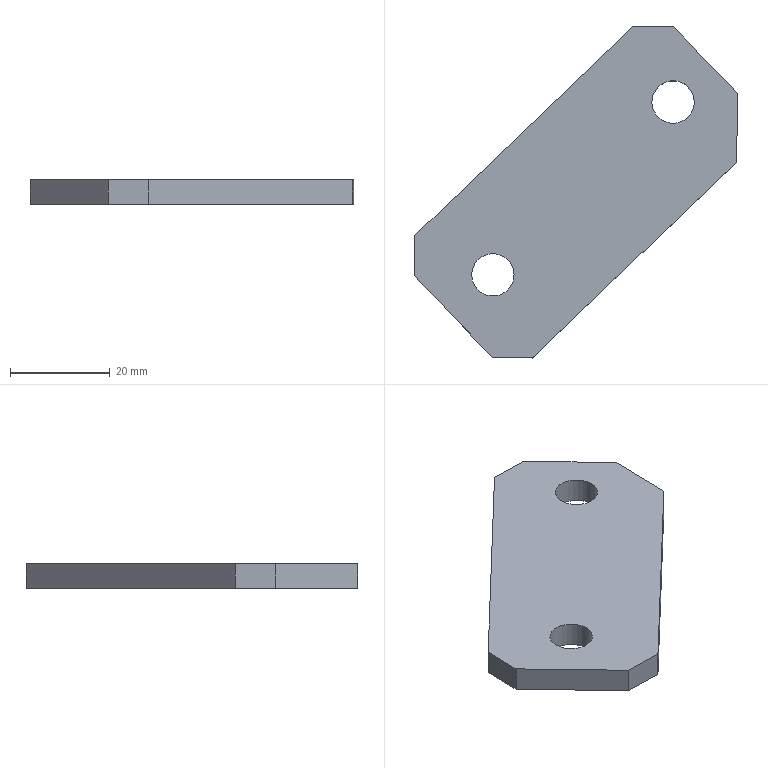Part | STEP file | gslz 2016.10.28-13_id1686_x_t | 1 solid | 12 faces | box 64.831 x 66.474 x 5 mm | volume 11193 mm3 | plane 10 | cylinder 2 | commonest cylinder face diameters 8.5 x2
STEP:
#1=CARTESIAN_POINT('',(0.,0.,0.));
#2=DIRECTION('',(0.,0.,1.));
#3=DIRECTION('',(1.,0.,0.));
#4=AXIS2_PLACEMENT_3D('',#1,#2,#3);
#5=CARTESIAN_POINT('',(590.854,-232.226,-99.));
#6=VERTEX_POINT('',#5);
#7=CARTESIAN_POINT('',(634.582,-190.292,-99.));
#8=VERTEX_POINT('',#7);
#9=CARTESIAN_POINT('',(426.204,-390.12,-99.));
#10=DIRECTION('',(0.7218,0.6921,0.));
#11=VECTOR('',#10,1.);
#12=LINE('',#9,#11);
#13=CARTESIAN_POINT('',(426.204,-390.12,-99.));
#14=DIRECTION('',(0.6921,-0.7218,0.));
#15=DIRECTION('',(0.7218,0.6921,0.));
#16=AXIS2_PLACEMENT_3D('',#13,#14,#15);
#17=PLANE('',#16);
#18=CARTESIAN_POINT('',(0.,0.));
#19=DIRECTION('',(1.,0.));
#20=VECTOR('',#19,1.);
#21=LINE('',#18,#20);
#22=(GEOMETRIC_REPRESENTATION_CONTEXT(2)PARAMETRIC_REPRESENTATION_CONTEXT()REPRESENTATION_CONTEXT('',''));
#23=DEFINITIONAL_REPRESENTATION('',(#21),#22);
#24=PCURVE('',#17,#23);
#25=CARTESIAN_POINT('',(467.733,-433.425,-99.));
#26=DIRECTION('',(0.,0.,1.));
#27=DIRECTION('',(1.,0.,0.));
#28=AXIS2_PLACEMENT_3D('',#25,#26,#27);
#29=PLANE('',#28);
#30=CARTESIAN_POINT('',(-41.529,43.306));
#31=DIRECTION('',(0.7218,0.6921));
#32=VECTOR('',#31,1.);
#33=LINE('',#30,#32);
#34=(GEOMETRIC_REPRESENTATION_CONTEXT(2)PARAMETRIC_REPRESENTATION_CONTEXT()REPRESENTATION_CONTEXT('',''));
#35=DEFINITIONAL_REPRESENTATION('',(#33),#34);
#36=PCURVE('',#29,#35);
#37=SURFACE_CURVE('',#12,(#24,#36),.PCURVE_S1.);
#38=EDGE_CURVE('',#6,#8,#37,.T.);
#39=ORIENTED_EDGE('',*,*,#38,.F.);
#40=CARTESIAN_POINT('',(590.854,-232.226,-94.));
#41=VERTEX_POINT('',#40);
#42=CARTESIAN_POINT('',(590.854,-232.226,-99.));
#43=DIRECTION('',(0.,0.,1.));
#44=VECTOR('',#43,1.);
#45=LINE('',#42,#44);
#46=CARTESIAN_POINT('',(228.122,0.));
#47=DIRECTION('',(0.,1.));
#48=VECTOR('',#47,1.);
#49=LINE('',#46,#48);
#50=(GEOMETRIC_REPRESENTATION_CONTEXT(2)PARAMETRIC_REPRESENTATION_CONTEXT()REPRESENTATION_CONTEXT('',''));
#51=DEFINITIONAL_REPRESENTATION('',(#49),#50);
#52=PCURVE('',#17,#51);
#53=CARTESIAN_POINT('',(590.858,-232.019,-99.));
#54=DIRECTION('',(0.9998,-0.02094,0.));
#55=DIRECTION('',(0.,0.,1.));
#56=AXIS2_PLACEMENT_3D('',#53,#54,#55);
#57=PLANE('',#56);
#58=CARTESIAN_POINT('',(0.,0.2071));
#59=DIRECTION('',(1.,0.));
#60=VECTOR('',#59,1.);
#61=LINE('',#58,#60);
#62=(GEOMETRIC_REPRESENTATION_CONTEXT(2)PARAMETRIC_REPRESENTATION_CONTEXT()REPRESENTATION_CONTEXT('',''));
#63=DEFINITIONAL_REPRESENTATION('',(#61),#62);
#64=PCURVE('',#57,#63);
#65=SURFACE_CURVE('',#45,(#52,#64),.PCURVE_S1.);
#66=EDGE_CURVE('',#6,#41,#65,.T.);
#67=ORIENTED_EDGE('',*,*,#66,.T.);
#68=CARTESIAN_POINT('',(634.582,-190.292,-94.));
#69=VERTEX_POINT('',#68);
#70=CARTESIAN_POINT('',(426.204,-390.12,-94.));
#71=DIRECTION('',(0.7218,0.6921,0.));
#72=VECTOR('',#71,1.);
#73=LINE('',#70,#72);
#74=CARTESIAN_POINT('',(0.,5.));
#75=DIRECTION('',(1.,0.));
#76=VECTOR('',#75,1.);
#77=LINE('',#74,#76);
#78=(GEOMETRIC_REPRESENTATION_CONTEXT(2)PARAMETRIC_REPRESENTATION_CONTEXT()REPRESENTATION_CONTEXT('',''));
#79=DEFINITIONAL_REPRESENTATION('',(#77),#78);
#80=PCURVE('',#17,#79);
#81=CARTESIAN_POINT('',(467.733,-433.425,-94.));
#82=DIRECTION('',(0.,0.,1.));
#83=DIRECTION('',(1.,0.,0.));
#84=AXIS2_PLACEMENT_3D('',#81,#82,#83);
#85=PLANE('',#84);
#86=CARTESIAN_POINT('',(-41.529,43.306));
#87=DIRECTION('',(0.7218,0.6921));
#88=VECTOR('',#87,1.);
#89=LINE('',#86,#88);
#90=(GEOMETRIC_REPRESENTATION_CONTEXT(2)PARAMETRIC_REPRESENTATION_CONTEXT()REPRESENTATION_CONTEXT('',''));
#91=DEFINITIONAL_REPRESENTATION('',(#89),#90);
#92=PCURVE('',#85,#91);
#93=SURFACE_CURVE('',#73,(#80,#92),.PCURVE_S1.);
#94=EDGE_CURVE('',#41,#69,#93,.T.);
#95=ORIENTED_EDGE('',*,*,#94,.T.);
#96=CARTESIAN_POINT('',(634.582,-190.292,-99.));
#97=DIRECTION('',(0.,0.,-1.));
#98=VECTOR('',#97,1.);
#99=LINE('',#96,#98);
#100=CARTESIAN_POINT('',(288.708,0.));
#101=DIRECTION('',(0.,-1.));
#102=VECTOR('',#101,1.);
#103=LINE('',#100,#102);
#104=(GEOMETRIC_REPRESENTATION_CONTEXT(2)PARAMETRIC_REPRESENTATION_CONTEXT()REPRESENTATION_CONTEXT('',''));
#105=DEFINITIONAL_REPRESENTATION('',(#103),#104);
#106=PCURVE('',#17,#105);
#107=CARTESIAN_POINT('',(642.859,-190.466,-99.));
#108=DIRECTION('',(0.02094,0.9998,0.));
#109=DIRECTION('',(0.,0.,-1.));
#110=AXIS2_PLACEMENT_3D('',#107,#108,#109);
#111=PLANE('',#110);
#112=CARTESIAN_POINT('',(0.,8.278));
#113=DIRECTION('',(1.,0.));
#114=VECTOR('',#113,1.);
#115=LINE('',#112,#114);
#116=(GEOMETRIC_REPRESENTATION_CONTEXT(2)PARAMETRIC_REPRESENTATION_CONTEXT()REPRESENTATION_CONTEXT('',''));
#117=DEFINITIONAL_REPRESENTATION('',(#115),#116);
#118=PCURVE('',#111,#117);
#119=SURFACE_CURVE('',#99,(#106,#118),.PCURVE_S1.);
#120=EDGE_CURVE('',#69,#8,#119,.T.);
#121=ORIENTED_EDGE('',*,*,#120,.T.);
#122=EDGE_LOOP('',(#39,#67,#95,#121));
#123=FACE_BOUND('',#122,.T.);
#124=ADVANCED_FACE('',(#123),#17,.F.);
#125=CARTESIAN_POINT('',(655.516,-203.876,-94.));
#126=VERTEX_POINT('',#125);
#127=CARTESIAN_POINT('',(642.652,-190.461,-94.));
#128=VERTEX_POINT('',#127);
#129=CARTESIAN_POINT('',(680.23,-229.648,-94.));
#130=DIRECTION('',(-0.6921,0.7218,0.));
#131=VECTOR('',#130,1.);
#132=LINE('',#129,#131);
#133=CARTESIAN_POINT('',(680.23,-229.648,-99.));
#134=DIRECTION('',(0.7218,0.6921,0.));
#135=DIRECTION('',(-0.6921,0.7218,0.));
#136=AXIS2_PLACEMENT_3D('',#133,#134,#135);
#137=PLANE('',#136);
#138=CARTESIAN_POINT('',(0.,5.));
#139=DIRECTION('',(1.,0.));
#140=VECTOR('',#139,1.);
#141=LINE('',#138,#140);
#142=(GEOMETRIC_REPRESENTATION_CONTEXT(2)PARAMETRIC_REPRESENTATION_CONTEXT()REPRESENTATION_CONTEXT('',''));
#143=DEFINITIONAL_REPRESENTATION('',(#141),#142);
#144=PCURVE('',#137,#143);
#145=CARTESIAN_POINT('',(212.497,203.778));
#146=DIRECTION('',(-0.6921,0.7218));
#147=VECTOR('',#146,1.);
#148=LINE('',#145,#147);
#149=(GEOMETRIC_REPRESENTATION_CONTEXT(2)PARAMETRIC_REPRESENTATION_CONTEXT()REPRESENTATION_CONTEXT('',''));
#150=DEFINITIONAL_REPRESENTATION('',(#148),#149);
#151=PCURVE('',#85,#150);
#152=SURFACE_CURVE('',#132,(#144,#151),.PCURVE_S1.);
#153=EDGE_CURVE('',#126,#128,#152,.T.);
#154=ORIENTED_EDGE('',*,*,#153,.F.);
#155=CARTESIAN_POINT('',(655.516,-203.876,-99.));
#156=VERTEX_POINT('',#155);
#157=CARTESIAN_POINT('',(655.516,-203.876,-99.));
#158=DIRECTION('',(0.,0.,-1.));
#159=VECTOR('',#158,1.);
#160=LINE('',#157,#159);
#161=CARTESIAN_POINT('',(35.707,0.));
#162=DIRECTION('',(0.,-1.));
#163=VECTOR('',#162,1.);
#164=LINE('',#161,#163);
#165=(GEOMETRIC_REPRESENTATION_CONTEXT(2)PARAMETRIC_REPRESENTATION_CONTEXT()REPRESENTATION_CONTEXT('',''));
#166=DEFINITIONAL_REPRESENTATION('',(#164),#165);
#167=PCURVE('',#137,#166);
#168=CARTESIAN_POINT('',(655.224,-217.808,-99.));
#169=DIRECTION('',(-0.9998,0.02094,0.));
#170=DIRECTION('',(0.,0.,1.));
#171=AXIS2_PLACEMENT_3D('',#168,#169,#170);
#172=PLANE('',#171);
#173=CARTESIAN_POINT('',(0.,13.935));
#174=DIRECTION('',(-1.,0.));
#175=VECTOR('',#174,1.);
#176=LINE('',#173,#175);
#177=(GEOMETRIC_REPRESENTATION_CONTEXT(2)PARAMETRIC_REPRESENTATION_CONTEXT()REPRESENTATION_CONTEXT('',''));
#178=DEFINITIONAL_REPRESENTATION('',(#176),#177);
#179=PCURVE('',#172,#178);
#180=SURFACE_CURVE('',#160,(#167,#179),.PCURVE_S1.);
#181=EDGE_CURVE('',#126,#156,#180,.T.);
#182=ORIENTED_EDGE('',*,*,#181,.T.);
#183=CARTESIAN_POINT('',(642.652,-190.461,-99.));
#184=VERTEX_POINT('',#183);
#185=CARTESIAN_POINT('',(680.23,-229.648,-99.));
#186=DIRECTION('',(-0.6921,0.7218,0.));
#187=VECTOR('',#186,1.);
#188=LINE('',#185,#187);
#189=CARTESIAN_POINT('',(0.,0.));
#190=DIRECTION('',(1.,0.));
#191=VECTOR('',#190,1.);
#192=LINE('',#189,#191);
#193=(GEOMETRIC_REPRESENTATION_CONTEXT(2)PARAMETRIC_REPRESENTATION_CONTEXT()REPRESENTATION_CONTEXT('',''));
#194=DEFINITIONAL_REPRESENTATION('',(#192),#193);
#195=PCURVE('',#137,#194);
#196=CARTESIAN_POINT('',(212.497,203.778));
#197=DIRECTION('',(-0.6921,0.7218));
#198=VECTOR('',#197,1.);
#199=LINE('',#196,#198);
#200=(GEOMETRIC_REPRESENTATION_CONTEXT(2)PARAMETRIC_REPRESENTATION_CONTEXT()REPRESENTATION_CONTEXT('',''));
#201=DEFINITIONAL_REPRESENTATION('',(#199),#200);
#202=PCURVE('',#29,#201);
#203=SURFACE_CURVE('',#188,(#195,#202),.PCURVE_S1.);
#204=EDGE_CURVE('',#156,#184,#203,.T.);
#205=ORIENTED_EDGE('',*,*,#204,.T.);
#206=CARTESIAN_POINT('',(642.652,-190.461,-99.));
#207=DIRECTION('',(0.,0.,1.));
#208=VECTOR('',#207,1.);
#209=LINE('',#206,#208);
#210=CARTESIAN_POINT('',(54.293,0.));
#211=DIRECTION('',(0.,1.));
#212=VECTOR('',#211,1.);
#213=LINE('',#210,#212);
#214=(GEOMETRIC_REPRESENTATION_CONTEXT(2)PARAMETRIC_REPRESENTATION_CONTEXT()REPRESENTATION_CONTEXT('',''));
#215=DEFINITIONAL_REPRESENTATION('',(#213),#214);
#216=PCURVE('',#137,#215);
#217=CARTESIAN_POINT('',(0.,0.2071));
#218=DIRECTION('',(-1.,0.));
#219=VECTOR('',#218,1.);
#220=LINE('',#217,#219);
#221=(GEOMETRIC_REPRESENTATION_CONTEXT(2)PARAMETRIC_REPRESENTATION_CONTEXT()REPRESENTATION_CONTEXT('',''));
#222=DEFINITIONAL_REPRESENTATION('',(#220),#221);
#223=PCURVE('',#111,#222);
#224=SURFACE_CURVE('',#209,(#216,#223),.PCURVE_S1.);
#225=EDGE_CURVE('',#184,#128,#224,.T.);
#226=ORIENTED_EDGE('',*,*,#225,.T.);
#227=EDGE_LOOP('',(#154,#182,#205,#226));
#228=FACE_BOUND('',#227,.T.);
#229=ADVANCED_FACE('',(#228),#137,.T.);
#230=CARTESIAN_POINT('',(614.387,-256.766,-99.));
#231=VERTEX_POINT('',#230);
#232=CARTESIAN_POINT('',(655.228,-217.601,-99.));
#233=VERTEX_POINT('',#232);
#234=CARTESIAN_POINT('',(449.737,-414.659,-99.));
#235=DIRECTION('',(0.7218,0.6921,0.));
#236=VECTOR('',#235,1.);
#237=LINE('',#234,#236);
#238=CARTESIAN_POINT('',(449.737,-414.659,-99.));
#239=DIRECTION('',(0.6921,-0.7218,0.));
#240=DIRECTION('',(0.7218,0.6921,0.));
#241=AXIS2_PLACEMENT_3D('',#238,#239,#240);
#242=PLANE('',#241);
#243=CARTESIAN_POINT('',(0.,0.));
#244=DIRECTION('',(1.,0.));
#245=VECTOR('',#244,1.);
#246=LINE('',#243,#245);
#247=(GEOMETRIC_REPRESENTATION_CONTEXT(2)PARAMETRIC_REPRESENTATION_CONTEXT()REPRESENTATION_CONTEXT('',''));
#248=DEFINITIONAL_REPRESENTATION('',(#246),#247);
#249=PCURVE('',#242,#248);
#250=CARTESIAN_POINT('',(-17.996,18.766));
#251=DIRECTION('',(0.7218,0.6921));
#252=VECTOR('',#251,1.);
#253=LINE('',#250,#252);
#254=(GEOMETRIC_REPRESENTATION_CONTEXT(2)PARAMETRIC_REPRESENTATION_CONTEXT()REPRESENTATION_CONTEXT('',''));
#255=DEFINITIONAL_REPRESENTATION('',(#253),#254);
#256=PCURVE('',#29,#255);
#257=SURFACE_CURVE('',#237,(#249,#256),.PCURVE_S1.);
#258=EDGE_CURVE('',#231,#233,#257,.T.);
#259=ORIENTED_EDGE('',*,*,#258,.T.);
#260=CARTESIAN_POINT('',(655.228,-217.601,-94.));
#261=VERTEX_POINT('',#260);
#262=CARTESIAN_POINT('',(655.228,-217.601,-99.));
#263=DIRECTION('',(0.,0.,1.));
#264=VECTOR('',#263,1.);
#265=LINE('',#262,#264);
#266=CARTESIAN_POINT('',(284.708,0.));
#267=DIRECTION('',(0.,1.));
#268=VECTOR('',#267,1.);
#269=LINE('',#266,#268);
#270=(GEOMETRIC_REPRESENTATION_CONTEXT(2)PARAMETRIC_REPRESENTATION_CONTEXT()REPRESENTATION_CONTEXT('',''));
#271=DEFINITIONAL_REPRESENTATION('',(#269),#270);
#272=PCURVE('',#242,#271);
#273=CARTESIAN_POINT('',(0.,0.2071));
#274=DIRECTION('',(1.,0.));
#275=VECTOR('',#274,1.);
#276=LINE('',#273,#275);
#277=(GEOMETRIC_REPRESENTATION_CONTEXT(2)PARAMETRIC_REPRESENTATION_CONTEXT()REPRESENTATION_CONTEXT('',''));
#278=DEFINITIONAL_REPRESENTATION('',(#276),#277);
#279=PCURVE('',#172,#278);
#280=SURFACE_CURVE('',#265,(#272,#279),.PCURVE_S1.);
#281=EDGE_CURVE('',#233,#261,#280,.T.);
#282=ORIENTED_EDGE('',*,*,#281,.T.);
#283=CARTESIAN_POINT('',(614.387,-256.766,-94.));
#284=VERTEX_POINT('',#283);
#285=CARTESIAN_POINT('',(449.737,-414.659,-94.));
#286=DIRECTION('',(0.7218,0.6921,0.));
#287=VECTOR('',#286,1.);
#288=LINE('',#285,#287);
#289=CARTESIAN_POINT('',(0.,5.));
#290=DIRECTION('',(1.,0.));
#291=VECTOR('',#290,1.);
#292=LINE('',#289,#291);
#293=(GEOMETRIC_REPRESENTATION_CONTEXT(2)PARAMETRIC_REPRESENTATION_CONTEXT()REPRESENTATION_CONTEXT('',''));
#294=DEFINITIONAL_REPRESENTATION('',(#292),#293);
#295=PCURVE('',#242,#294);
#296=CARTESIAN_POINT('',(-17.996,18.766));
#297=DIRECTION('',(0.7218,0.6921));
#298=VECTOR('',#297,1.);
#299=LINE('',#296,#298);
#300=(GEOMETRIC_REPRESENTATION_CONTEXT(2)PARAMETRIC_REPRESENTATION_CONTEXT()REPRESENTATION_CONTEXT('',''));
#301=DEFINITIONAL_REPRESENTATION('',(#299),#300);
#302=PCURVE('',#85,#301);
#303=SURFACE_CURVE('',#288,(#295,#302),.PCURVE_S1.);
#304=EDGE_CURVE('',#284,#261,#303,.T.);
#305=ORIENTED_EDGE('',*,*,#304,.F.);
#306=CARTESIAN_POINT('',(614.387,-256.766,-99.));
#307=DIRECTION('',(0.,0.,-1.));
#308=VECTOR('',#307,1.);
#309=LINE('',#306,#308);
#310=CARTESIAN_POINT('',(228.122,0.));
#311=DIRECTION('',(0.,-1.));
#312=VECTOR('',#311,1.);
#313=LINE('',#310,#312);
#314=(GEOMETRIC_REPRESENTATION_CONTEXT(2)PARAMETRIC_REPRESENTATION_CONTEXT()REPRESENTATION_CONTEXT('',''));
#315=DEFINITIONAL_REPRESENTATION('',(#313),#314);
#316=PCURVE('',#242,#315);
#317=CARTESIAN_POINT('',(606.11,-256.593,-99.));
#318=DIRECTION('',(-0.02094,-0.9998,0.));
#319=DIRECTION('',(0.,0.,-1.));
#320=AXIS2_PLACEMENT_3D('',#317,#318,#319);
#321=PLANE('',#320);
#322=CARTESIAN_POINT('',(0.,8.278));
#323=DIRECTION('',(1.,0.));
#324=VECTOR('',#323,1.);
#325=LINE('',#322,#324);
#326=(GEOMETRIC_REPRESENTATION_CONTEXT(2)PARAMETRIC_REPRESENTATION_CONTEXT()REPRESENTATION_CONTEXT('',''));
#327=DEFINITIONAL_REPRESENTATION('',(#325),#326);
#328=PCURVE('',#321,#327);
#329=SURFACE_CURVE('',#309,(#316,#328),.PCURVE_S1.);
#330=EDGE_CURVE('',#284,#231,#329,.T.);
#331=ORIENTED_EDGE('',*,*,#330,.T.);
#332=EDGE_LOOP('',(#259,#282,#305,#331));
#333=FACE_BOUND('',#332,.T.);
#334=ADVANCED_FACE('',(#333),#242,.T.);
#335=CARTESIAN_POINT('',(606.318,-256.597,-99.));
#336=VERTEX_POINT('',#335);
#337=CARTESIAN_POINT('',(590.685,-240.296,-99.));
#338=VERTEX_POINT('',#337);
#339=CARTESIAN_POINT('',(628.263,-279.482,-99.));
#340=DIRECTION('',(-0.6921,0.7218,0.));
#341=VECTOR('',#340,1.);
#342=LINE('',#339,#341);
#343=CARTESIAN_POINT('',(628.263,-279.482,-99.));
#344=DIRECTION('',(0.7218,0.6921,0.));
#345=DIRECTION('',(-0.6921,0.7218,0.));
#346=AXIS2_PLACEMENT_3D('',#343,#344,#345);
#347=PLANE('',#346);
#348=CARTESIAN_POINT('',(0.,0.));
#349=DIRECTION('',(1.,0.));
#350=VECTOR('',#349,1.);
#351=LINE('',#348,#350);
#352=(GEOMETRIC_REPRESENTATION_CONTEXT(2)PARAMETRIC_REPRESENTATION_CONTEXT()REPRESENTATION_CONTEXT('',''));
#353=DEFINITIONAL_REPRESENTATION('',(#351),#352);
#354=PCURVE('',#347,#353);
#355=CARTESIAN_POINT('',(160.531,153.943));
#356=DIRECTION('',(-0.6921,0.7218));
#357=VECTOR('',#356,1.);
#358=LINE('',#355,#357);
#359=(GEOMETRIC_REPRESENTATION_CONTEXT(2)PARAMETRIC_REPRESENTATION_CONTEXT()REPRESENTATION_CONTEXT('',''));
#360=DEFINITIONAL_REPRESENTATION('',(#358),#359);
#361=PCURVE('',#29,#360);
#362=SURFACE_CURVE('',#342,(#354,#361),.PCURVE_S1.);
#363=EDGE_CURVE('',#336,#338,#362,.T.);
#364=ORIENTED_EDGE('',*,*,#363,.F.);
#365=CARTESIAN_POINT('',(606.318,-256.597,-94.));
#366=VERTEX_POINT('',#365);
#367=CARTESIAN_POINT('',(606.318,-256.597,-99.));
#368=DIRECTION('',(0.,0.,1.));
#369=VECTOR('',#368,1.);
#370=LINE('',#367,#369);
#371=CARTESIAN_POINT('',(31.707,0.));
#372=DIRECTION('',(0.,1.));
#373=VECTOR('',#372,1.);
#374=LINE('',#371,#373);
#375=(GEOMETRIC_REPRESENTATION_CONTEXT(2)PARAMETRIC_REPRESENTATION_CONTEXT()REPRESENTATION_CONTEXT('',''));
#376=DEFINITIONAL_REPRESENTATION('',(#374),#375);
#377=PCURVE('',#347,#376);
#378=CARTESIAN_POINT('',(0.,0.2071));
#379=DIRECTION('',(-1.,0.));
#380=VECTOR('',#379,1.);
#381=LINE('',#378,#380);
#382=(GEOMETRIC_REPRESENTATION_CONTEXT(2)PARAMETRIC_REPRESENTATION_CONTEXT()REPRESENTATION_CONTEXT('',''));
#383=DEFINITIONAL_REPRESENTATION('',(#381),#382);
#384=PCURVE('',#321,#383);
#385=SURFACE_CURVE('',#370,(#377,#384),.PCURVE_S1.);
#386=EDGE_CURVE('',#336,#366,#385,.T.);
#387=ORIENTED_EDGE('',*,*,#386,.T.);
#388=CARTESIAN_POINT('',(590.685,-240.296,-94.));
#389=VERTEX_POINT('',#388);
#390=CARTESIAN_POINT('',(628.263,-279.482,-94.));
#391=DIRECTION('',(-0.6921,0.7218,0.));
#392=VECTOR('',#391,1.);
#393=LINE('',#390,#392);
#394=CARTESIAN_POINT('',(0.,5.));
#395=DIRECTION('',(1.,0.));
#396=VECTOR('',#395,1.);
#397=LINE('',#394,#396);
#398=(GEOMETRIC_REPRESENTATION_CONTEXT(2)PARAMETRIC_REPRESENTATION_CONTEXT()REPRESENTATION_CONTEXT('',''));
#399=DEFINITIONAL_REPRESENTATION('',(#397),#398);
#400=PCURVE('',#347,#399);
#401=CARTESIAN_POINT('',(160.531,153.943));
#402=DIRECTION('',(-0.6921,0.7218));
#403=VECTOR('',#402,1.);
#404=LINE('',#401,#403);
#405=(GEOMETRIC_REPRESENTATION_CONTEXT(2)PARAMETRIC_REPRESENTATION_CONTEXT()REPRESENTATION_CONTEXT('',''));
#406=DEFINITIONAL_REPRESENTATION('',(#404),#405);
#407=PCURVE('',#85,#406);
#408=SURFACE_CURVE('',#393,(#400,#407),.PCURVE_S1.);
#409=EDGE_CURVE('',#366,#389,#408,.T.);
#410=ORIENTED_EDGE('',*,*,#409,.T.);
#411=CARTESIAN_POINT('',(590.685,-240.296,-99.));
#412=DIRECTION('',(0.,0.,-1.));
#413=VECTOR('',#412,1.);
#414=LINE('',#411,#413);
#415=CARTESIAN_POINT('',(54.293,0.));
#416=DIRECTION('',(0.,-1.));
#417=VECTOR('',#416,1.);
#418=LINE('',#415,#417);
#419=(GEOMETRIC_REPRESENTATION_CONTEXT(2)PARAMETRIC_REPRESENTATION_CONTEXT()REPRESENTATION_CONTEXT('',''));
#420=DEFINITIONAL_REPRESENTATION('',(#418),#419);
#421=PCURVE('',#347,#420);
#422=CARTESIAN_POINT('',(0.,8.278));
#423=DIRECTION('',(-1.,0.));
#424=VECTOR('',#423,1.);
#425=LINE('',#422,#424);
#426=(GEOMETRIC_REPRESENTATION_CONTEXT(2)PARAMETRIC_REPRESENTATION_CONTEXT()REPRESENTATION_CONTEXT('',''));
#427=DEFINITIONAL_REPRESENTATION('',(#425),#426);
#428=PCURVE('',#57,#427);
#429=SURFACE_CURVE('',#414,(#421,#428),.PCURVE_S1.);
#430=EDGE_CURVE('',#389,#338,#429,.T.);
#431=ORIENTED_EDGE('',*,*,#430,.T.);
#432=EDGE_LOOP('',(#364,#387,#410,#431));
#433=FACE_BOUND('',#432,.T.);
#434=ADVANCED_FACE('',(#433),#347,.F.);
#435=CARTESIAN_POINT('',(610.705,-240.126,-99.));
#436=VERTEX_POINT('',#435);
#437=CARTESIAN_POINT('',(606.455,-240.126,-99.));
#438=DIRECTION('',(0.,0.,-1.));
#439=DIRECTION('',(1.,0.,0.));
#440=AXIS2_PLACEMENT_3D('',#437,#438,#439);
#441=CIRCLE('',#440,4.25);
#442=CARTESIAN_POINT('',(606.455,-240.126,-99.));
#443=DIRECTION('',(0.,0.,1.));
#444=DIRECTION('',(1.,0.,0.));
#445=AXIS2_PLACEMENT_3D('',#442,#443,#444);
#446=CYLINDRICAL_SURFACE('',#445,4.25);
#447=CARTESIAN_POINT('',(6.283,0.));
#448=DIRECTION('',(-1.,0.));
#449=VECTOR('',#448,1.);
#450=LINE('',#447,#449);
#451=(GEOMETRIC_REPRESENTATION_CONTEXT(2)PARAMETRIC_REPRESENTATION_CONTEXT()REPRESENTATION_CONTEXT('',''));
#452=DEFINITIONAL_REPRESENTATION('',(#450),#451);
#453=PCURVE('',#446,#452);
#454=CARTESIAN_POINT('',(142.973,193.299));
#455=CARTESIAN_POINT('',(142.973,185.938));
#456=CARTESIAN_POINT('',(136.598,189.619));
#457=CARTESIAN_POINT('',(130.223,193.299));
#458=CARTESIAN_POINT('',(136.598,196.98));
#459=CARTESIAN_POINT('',(142.973,200.661));
#460=CARTESIAN_POINT('',(142.973,193.299));
#461=(BOUNDED_CURVE()B_SPLINE_CURVE(2,(#454,#455,#456,#457,#458,#459,#460),.UNSPECIFIED.,.T.,.F.)B_SPLINE_CURVE_WITH_KNOTS((1,2,2,2,2,1),(-2.094,0.,2.094,4.189,6.283,8.378),.UNSPECIFIED.)CURVE()GEOMETRIC_REPRESENTATION_ITEM()RATIONAL_B_SPLINE_CURVE((1.,0.5,1.,0.5,1.,0.5,1.))REPRESENTATION_ITEM(''));
#462=(GEOMETRIC_REPRESENTATION_CONTEXT(2)PARAMETRIC_REPRESENTATION_CONTEXT()REPRESENTATION_CONTEXT('',''));
#463=DEFINITIONAL_REPRESENTATION('',(#461),#462);
#464=PCURVE('',#29,#463);
#465=SURFACE_CURVE('',#441,(#453,#464),.PCURVE_S1.);
#466=EDGE_CURVE('',#436,#436,#465,.T.);
#467=ORIENTED_EDGE('',*,*,#466,.F.);
#468=CARTESIAN_POINT('',(610.705,-240.126,-94.));
#469=VERTEX_POINT('',#468);
#470=CARTESIAN_POINT('',(610.705,-240.126,-99.));
#471=CARTESIAN_POINT('',(610.705,-240.126,-94.));
#472=B_SPLINE_CURVE_WITH_KNOTS('',1,(#470,#471),.UNSPECIFIED.,.F.,.F.,(2,2),(0.,5.),.PIECEWISE_BEZIER_KNOTS.);
#473=CARTESIAN_POINT('',(6.283,0.));
#474=DIRECTION('',(0.,1.));
#475=VECTOR('',#474,1.);
#476=LINE('',#473,#475);
#477=(GEOMETRIC_REPRESENTATION_CONTEXT(2)PARAMETRIC_REPRESENTATION_CONTEXT()REPRESENTATION_CONTEXT('',''));
#478=DEFINITIONAL_REPRESENTATION('',(#476),#477);
#479=PCURVE('',#446,#478);
#480=CARTESIAN_POINT('',(0.,0.));
#481=DIRECTION('',(0.,1.));
#482=VECTOR('',#481,1.);
#483=LINE('',#480,#482);
#484=(GEOMETRIC_REPRESENTATION_CONTEXT(2)PARAMETRIC_REPRESENTATION_CONTEXT()REPRESENTATION_CONTEXT('',''));
#485=DEFINITIONAL_REPRESENTATION('',(#483),#484);
#486=PCURVE('',#446,#485);
#487=SEAM_CURVE('',#472,(#479,#486),.PCURVE_S1.);
#488=EDGE_CURVE('',#436,#469,#487,.T.);
#489=ORIENTED_EDGE('',*,*,#488,.T.);
#490=CARTESIAN_POINT('',(606.455,-240.126,-94.));
#491=DIRECTION('',(0.,0.,-1.));
#492=DIRECTION('',(1.,0.,0.));
#493=AXIS2_PLACEMENT_3D('',#490,#491,#492);
#494=CIRCLE('',#493,4.25);
#495=CARTESIAN_POINT('',(6.283,5.));
#496=DIRECTION('',(-1.,0.));
#497=VECTOR('',#496,1.);
#498=LINE('',#495,#497);
#499=(GEOMETRIC_REPRESENTATION_CONTEXT(2)PARAMETRIC_REPRESENTATION_CONTEXT()REPRESENTATION_CONTEXT('',''));
#500=DEFINITIONAL_REPRESENTATION('',(#498),#499);
#501=PCURVE('',#446,#500);
#502=CARTESIAN_POINT('',(142.973,193.299));
#503=CARTESIAN_POINT('',(142.973,185.938));
#504=CARTESIAN_POINT('',(136.598,189.619));
#505=CARTESIAN_POINT('',(130.223,193.299));
#506=CARTESIAN_POINT('',(136.598,196.98));
#507=CARTESIAN_POINT('',(142.973,200.661));
#508=CARTESIAN_POINT('',(142.973,193.299));
#509=(BOUNDED_CURVE()B_SPLINE_CURVE(2,(#502,#503,#504,#505,#506,#507,#508),.UNSPECIFIED.,.T.,.F.)B_SPLINE_CURVE_WITH_KNOTS((1,2,2,2,2,1),(-2.094,0.,2.094,4.189,6.283,8.378),.UNSPECIFIED.)CURVE()GEOMETRIC_REPRESENTATION_ITEM()RATIONAL_B_SPLINE_CURVE((1.,0.5,1.,0.5,1.,0.5,1.))REPRESENTATION_ITEM(''));
#510=(GEOMETRIC_REPRESENTATION_CONTEXT(2)PARAMETRIC_REPRESENTATION_CONTEXT()REPRESENTATION_CONTEXT('',''));
#511=DEFINITIONAL_REPRESENTATION('',(#509),#510);
#512=PCURVE('',#85,#511);
#513=SURFACE_CURVE('',#494,(#501,#512),.PCURVE_S1.);
#514=EDGE_CURVE('',#469,#469,#513,.T.);
#515=ORIENTED_EDGE('',*,*,#514,.T.);
#516=ORIENTED_EDGE('',*,*,#488,.F.);
#517=EDGE_LOOP('',(#467,#489,#515,#516));
#518=FACE_BOUND('',#517,.F.);
#519=ADVANCED_FACE('',(#518),#446,.F.);
#520=CARTESIAN_POINT('',(646.793,-205.519,-99.));
#521=VERTEX_POINT('',#520);
#522=CARTESIAN_POINT('',(642.543,-205.519,-99.));
#523=DIRECTION('',(0.,0.,-1.));
#524=DIRECTION('',(1.,0.,0.));
#525=AXIS2_PLACEMENT_3D('',#522,#523,#524);
#526=CIRCLE('',#525,4.25);
#527=CARTESIAN_POINT('',(642.543,-205.519,-99.));
#528=DIRECTION('',(0.,0.,1.));
#529=DIRECTION('',(1.,0.,0.));
#530=AXIS2_PLACEMENT_3D('',#527,#528,#529);
#531=CYLINDRICAL_SURFACE('',#530,4.25);
#532=CARTESIAN_POINT('',(6.283,0.));
#533=DIRECTION('',(-1.,0.));
#534=VECTOR('',#533,1.);
#535=LINE('',#532,#534);
#536=(GEOMETRIC_REPRESENTATION_CONTEXT(2)PARAMETRIC_REPRESENTATION_CONTEXT()REPRESENTATION_CONTEXT('',''));
#537=DEFINITIONAL_REPRESENTATION('',(#535),#536);
#538=PCURVE('',#531,#537);
#539=CARTESIAN_POINT('',(179.061,227.907));
#540=CARTESIAN_POINT('',(179.061,220.545));
#541=CARTESIAN_POINT('',(172.686,224.226));
#542=CARTESIAN_POINT('',(166.311,227.907));
#543=CARTESIAN_POINT('',(172.686,231.587));
#544=CARTESIAN_POINT('',(179.061,235.268));
#545=CARTESIAN_POINT('',(179.061,227.907));
#546=(BOUNDED_CURVE()B_SPLINE_CURVE(2,(#539,#540,#541,#542,#543,#544,#545),.UNSPECIFIED.,.T.,.F.)B_SPLINE_CURVE_WITH_KNOTS((1,2,2,2,2,1),(-2.094,0.,2.094,4.189,6.283,8.378),.UNSPECIFIED.)CURVE()GEOMETRIC_REPRESENTATION_ITEM()RATIONAL_B_SPLINE_CURVE((1.,0.5,1.,0.5,1.,0.5,1.))REPRESENTATION_ITEM(''));
#547=(GEOMETRIC_REPRESENTATION_CONTEXT(2)PARAMETRIC_REPRESENTATION_CONTEXT()REPRESENTATION_CONTEXT('',''));
#548=DEFINITIONAL_REPRESENTATION('',(#546),#547);
#549=PCURVE('',#29,#548);
#550=SURFACE_CURVE('',#526,(#538,#549),.PCURVE_S1.);
#551=EDGE_CURVE('',#521,#521,#550,.T.);
#552=ORIENTED_EDGE('',*,*,#551,.F.);
#553=CARTESIAN_POINT('',(646.793,-205.519,-94.));
#554=VERTEX_POINT('',#553);
#555=CARTESIAN_POINT('',(646.793,-205.519,-99.));
#556=CARTESIAN_POINT('',(646.793,-205.519,-94.));
#557=B_SPLINE_CURVE_WITH_KNOTS('',1,(#555,#556),.UNSPECIFIED.,.F.,.F.,(2,2),(0.,5.),.PIECEWISE_BEZIER_KNOTS.);
#558=CARTESIAN_POINT('',(6.283,0.));
#559=DIRECTION('',(0.,1.));
#560=VECTOR('',#559,1.);
#561=LINE('',#558,#560);
#562=(GEOMETRIC_REPRESENTATION_CONTEXT(2)PARAMETRIC_REPRESENTATION_CONTEXT()REPRESENTATION_CONTEXT('',''));
#563=DEFINITIONAL_REPRESENTATION('',(#561),#562);
#564=PCURVE('',#531,#563);
#565=CARTESIAN_POINT('',(0.,0.));
#566=DIRECTION('',(0.,1.));
#567=VECTOR('',#566,1.);
#568=LINE('',#565,#567);
#569=(GEOMETRIC_REPRESENTATION_CONTEXT(2)PARAMETRIC_REPRESENTATION_CONTEXT()REPRESENTATION_CONTEXT('',''));
#570=DEFINITIONAL_REPRESENTATION('',(#568),#569);
#571=PCURVE('',#531,#570);
#572=SEAM_CURVE('',#557,(#564,#571),.PCURVE_S1.);
#573=EDGE_CURVE('',#521,#554,#572,.T.);
#574=ORIENTED_EDGE('',*,*,#573,.T.);
#575=CARTESIAN_POINT('',(642.543,-205.519,-94.));
#576=DIRECTION('',(0.,0.,-1.));
#577=DIRECTION('',(1.,0.,0.));
#578=AXIS2_PLACEMENT_3D('',#575,#576,#577);
#579=CIRCLE('',#578,4.25);
#580=CARTESIAN_POINT('',(6.283,5.));
#581=DIRECTION('',(-1.,0.));
#582=VECTOR('',#581,1.);
#583=LINE('',#580,#582);
#584=(GEOMETRIC_REPRESENTATION_CONTEXT(2)PARAMETRIC_REPRESENTATION_CONTEXT()REPRESENTATION_CONTEXT('',''));
#585=DEFINITIONAL_REPRESENTATION('',(#583),#584);
#586=PCURVE('',#531,#585);
#587=CARTESIAN_POINT('',(179.061,227.907));
#588=CARTESIAN_POINT('',(179.061,220.545));
#589=CARTESIAN_POINT('',(172.686,224.226));
#590=CARTESIAN_POINT('',(166.311,227.907));
#591=CARTESIAN_POINT('',(172.686,231.587));
#592=CARTESIAN_POINT('',(179.061,235.268));
#593=CARTESIAN_POINT('',(179.061,227.907));
#594=(BOUNDED_CURVE()B_SPLINE_CURVE(2,(#587,#588,#589,#590,#591,#592,#593),.UNSPECIFIED.,.T.,.F.)B_SPLINE_CURVE_WITH_KNOTS((1,2,2,2,2,1),(-2.094,0.,2.094,4.189,6.283,8.378),.UNSPECIFIED.)CURVE()GEOMETRIC_REPRESENTATION_ITEM()RATIONAL_B_SPLINE_CURVE((1.,0.5,1.,0.5,1.,0.5,1.))REPRESENTATION_ITEM(''));
#595=(GEOMETRIC_REPRESENTATION_CONTEXT(2)PARAMETRIC_REPRESENTATION_CONTEXT()REPRESENTATION_CONTEXT('',''));
#596=DEFINITIONAL_REPRESENTATION('',(#594),#595);
#597=PCURVE('',#85,#596);
#598=SURFACE_CURVE('',#579,(#586,#597),.PCURVE_S1.);
#599=EDGE_CURVE('',#554,#554,#598,.T.);
#600=ORIENTED_EDGE('',*,*,#599,.T.);
#601=ORIENTED_EDGE('',*,*,#573,.F.);
#602=EDGE_LOOP('',(#552,#574,#600,#601));
#603=FACE_BOUND('',#602,.F.);
#604=ADVANCED_FACE('',(#603),#531,.F.);
#605=ORIENTED_EDGE('',*,*,#466,.F.);
#606=EDGE_LOOP('',(#605));
#607=FACE_BOUND('',#606,.T.);
#608=ORIENTED_EDGE('',*,*,#204,.F.);
#609=CARTESIAN_POINT('',(655.224,-217.808,-99.));
#610=DIRECTION('',(-0.02094,-0.9998,0.));
#611=VECTOR('',#610,1.);
#612=LINE('',#609,#611);
#613=CARTESIAN_POINT('',(187.491,215.618));
#614=DIRECTION('',(-0.02094,-0.9998));
#615=VECTOR('',#614,1.);
#616=LINE('',#613,#615);
#617=(GEOMETRIC_REPRESENTATION_CONTEXT(2)PARAMETRIC_REPRESENTATION_CONTEXT()REPRESENTATION_CONTEXT('',''));
#618=DEFINITIONAL_REPRESENTATION('',(#616),#617);
#619=PCURVE('',#29,#618);
#620=CARTESIAN_POINT('',(0.,0.));
#621=DIRECTION('',(0.,-1.));
#622=VECTOR('',#621,1.);
#623=LINE('',#620,#622);
#624=(GEOMETRIC_REPRESENTATION_CONTEXT(2)PARAMETRIC_REPRESENTATION_CONTEXT()REPRESENTATION_CONTEXT('',''));
#625=DEFINITIONAL_REPRESENTATION('',(#623),#624);
#626=PCURVE('',#172,#625);
#627=SURFACE_CURVE('',#612,(#619,#626),.PCURVE_S1.);
#628=EDGE_CURVE('',#156,#233,#627,.T.);
#629=ORIENTED_EDGE('',*,*,#628,.T.);
#630=ORIENTED_EDGE('',*,*,#258,.F.);
#631=CARTESIAN_POINT('',(606.11,-256.593,-99.));
#632=DIRECTION('',(-0.9998,0.02094,0.));
#633=VECTOR('',#632,1.);
#634=LINE('',#631,#633);
#635=CARTESIAN_POINT('',(138.378,176.833));
#636=DIRECTION('',(-0.9998,0.02094));
#637=VECTOR('',#636,1.);
#638=LINE('',#635,#637);
#639=(GEOMETRIC_REPRESENTATION_CONTEXT(2)PARAMETRIC_REPRESENTATION_CONTEXT()REPRESENTATION_CONTEXT('',''));
#640=DEFINITIONAL_REPRESENTATION('',(#638),#639);
#641=PCURVE('',#29,#640);
#642=CARTESIAN_POINT('',(0.,0.));
#643=DIRECTION('',(0.,-1.));
#644=VECTOR('',#643,1.);
#645=LINE('',#642,#644);
#646=(GEOMETRIC_REPRESENTATION_CONTEXT(2)PARAMETRIC_REPRESENTATION_CONTEXT()REPRESENTATION_CONTEXT('',''));
#647=DEFINITIONAL_REPRESENTATION('',(#645),#646);
#648=PCURVE('',#321,#647);
#649=SURFACE_CURVE('',#634,(#641,#648),.PCURVE_S1.);
#650=EDGE_CURVE('',#231,#336,#649,.T.);
#651=ORIENTED_EDGE('',*,*,#650,.T.);
#652=ORIENTED_EDGE('',*,*,#363,.T.);
#653=CARTESIAN_POINT('',(590.858,-232.019,-99.));
#654=DIRECTION('',(0.02094,0.9998,0.));
#655=VECTOR('',#654,1.);
#656=LINE('',#653,#655);
#657=CARTESIAN_POINT('',(123.125,201.406));
#658=DIRECTION('',(0.02094,0.9998));
#659=VECTOR('',#658,1.);
#660=LINE('',#657,#659);
#661=(GEOMETRIC_REPRESENTATION_CONTEXT(2)PARAMETRIC_REPRESENTATION_CONTEXT()REPRESENTATION_CONTEXT('',''));
#662=DEFINITIONAL_REPRESENTATION('',(#660),#661);
#663=PCURVE('',#29,#662);
#664=CARTESIAN_POINT('',(0.,0.));
#665=DIRECTION('',(0.,-1.));
#666=VECTOR('',#665,1.);
#667=LINE('',#664,#666);
#668=(GEOMETRIC_REPRESENTATION_CONTEXT(2)PARAMETRIC_REPRESENTATION_CONTEXT()REPRESENTATION_CONTEXT('',''));
#669=DEFINITIONAL_REPRESENTATION('',(#667),#668);
#670=PCURVE('',#57,#669);
#671=SURFACE_CURVE('',#656,(#663,#670),.PCURVE_S1.);
#672=EDGE_CURVE('',#338,#6,#671,.T.);
#673=ORIENTED_EDGE('',*,*,#672,.T.);
#674=ORIENTED_EDGE('',*,*,#38,.T.);
#675=CARTESIAN_POINT('',(642.859,-190.466,-99.));
#676=DIRECTION('',(0.9998,-0.02094,0.));
#677=VECTOR('',#676,1.);
#678=LINE('',#675,#677);
#679=CARTESIAN_POINT('',(175.126,242.96));
#680=DIRECTION('',(0.9998,-0.02094));
#681=VECTOR('',#680,1.);
#682=LINE('',#679,#681);
#683=(GEOMETRIC_REPRESENTATION_CONTEXT(2)PARAMETRIC_REPRESENTATION_CONTEXT()REPRESENTATION_CONTEXT('',''));
#684=DEFINITIONAL_REPRESENTATION('',(#682),#683);
#685=PCURVE('',#29,#684);
#686=CARTESIAN_POINT('',(0.,0.));
#687=DIRECTION('',(0.,-1.));
#688=VECTOR('',#687,1.);
#689=LINE('',#686,#688);
#690=(GEOMETRIC_REPRESENTATION_CONTEXT(2)PARAMETRIC_REPRESENTATION_CONTEXT()REPRESENTATION_CONTEXT('',''));
#691=DEFINITIONAL_REPRESENTATION('',(#689),#690);
#692=PCURVE('',#111,#691);
#693=SURFACE_CURVE('',#678,(#685,#692),.PCURVE_S1.);
#694=EDGE_CURVE('',#8,#184,#693,.T.);
#695=ORIENTED_EDGE('',*,*,#694,.T.);
#696=EDGE_LOOP('',(#608,#629,#630,#651,#652,#673,#674,#695));
#697=FACE_BOUND('',#696,.T.);
#698=ORIENTED_EDGE('',*,*,#551,.F.);
#699=EDGE_LOOP('',(#698));
#700=FACE_BOUND('',#699,.T.);
#701=ADVANCED_FACE('',(#607,#697,#700),#29,.F.);
#702=ORIENTED_EDGE('',*,*,#514,.T.);
#703=EDGE_LOOP('',(#702));
#704=FACE_BOUND('',#703,.T.);
#705=ORIENTED_EDGE('',*,*,#304,.T.);
#706=CARTESIAN_POINT('',(650.627,-437.256,-94.));
#707=DIRECTION('',(0.02094,0.9998,0.));
#708=VECTOR('',#707,1.);
#709=LINE('',#706,#708);
#710=CARTESIAN_POINT('',(182.894,-3.831));
#711=DIRECTION('',(0.02094,0.9998));
#712=VECTOR('',#711,1.);
#713=LINE('',#710,#712);
#714=(GEOMETRIC_REPRESENTATION_CONTEXT(2)PARAMETRIC_REPRESENTATION_CONTEXT()REPRESENTATION_CONTEXT('',''));
#715=DEFINITIONAL_REPRESENTATION('',(#713),#714);
#716=PCURVE('',#85,#715);
#717=CARTESIAN_POINT('',(5.,-219.497));
#718=DIRECTION('',(0.,1.));
#719=VECTOR('',#718,1.);
#720=LINE('',#717,#719);
#721=(GEOMETRIC_REPRESENTATION_CONTEXT(2)PARAMETRIC_REPRESENTATION_CONTEXT()REPRESENTATION_CONTEXT('',''));
#722=DEFINITIONAL_REPRESENTATION('',(#720),#721);
#723=PCURVE('',#172,#722);
#724=SURFACE_CURVE('',#709,(#716,#723),.PCURVE_S1.);
#725=EDGE_CURVE('',#261,#126,#724,.T.);
#726=ORIENTED_EDGE('',*,*,#725,.T.);
#727=ORIENTED_EDGE('',*,*,#153,.T.);
#728=CARTESIAN_POINT('',(471.483,-186.876,-94.));
#729=DIRECTION('',(-0.9998,0.02094,0.));
#730=VECTOR('',#729,1.);
#731=LINE('',#728,#730);
#732=CARTESIAN_POINT('',(3.75,246.549));
#733=DIRECTION('',(-0.9998,0.02094));
#734=VECTOR('',#733,1.);
#735=LINE('',#732,#734);
#736=(GEOMETRIC_REPRESENTATION_CONTEXT(2)PARAMETRIC_REPRESENTATION_CONTEXT()REPRESENTATION_CONTEXT('',''));
#737=DEFINITIONAL_REPRESENTATION('',(#735),#736);
#738=PCURVE('',#85,#737);
#739=CARTESIAN_POINT('',(-5.,171.414));
#740=DIRECTION('',(0.,1.));
#741=VECTOR('',#740,1.);
#742=LINE('',#739,#741);
#743=(GEOMETRIC_REPRESENTATION_CONTEXT(2)PARAMETRIC_REPRESENTATION_CONTEXT()REPRESENTATION_CONTEXT('',''));
#744=DEFINITIONAL_REPRESENTATION('',(#742),#743);
#745=PCURVE('',#111,#744);
#746=SURFACE_CURVE('',#731,(#738,#745),.PCURVE_S1.);
#747=EDGE_CURVE('',#128,#69,#746,.T.);
#748=ORIENTED_EDGE('',*,*,#747,.T.);
#749=ORIENTED_EDGE('',*,*,#94,.F.);
#750=CARTESIAN_POINT('',(586.617,-434.501,-94.));
#751=DIRECTION('',(-0.02094,-0.9998,0.));
#752=VECTOR('',#751,1.);
#753=LINE('',#750,#752);
#754=CARTESIAN_POINT('',(118.884,-1.076));
#755=DIRECTION('',(-0.02094,-0.9998));
#756=VECTOR('',#755,1.);
#757=LINE('',#754,#756);
#758=(GEOMETRIC_REPRESENTATION_CONTEXT(2)PARAMETRIC_REPRESENTATION_CONTEXT()REPRESENTATION_CONTEXT('',''));
#759=DEFINITIONAL_REPRESENTATION('',(#757),#758);
#760=PCURVE('',#85,#759);
#761=CARTESIAN_POINT('',(5.,202.526));
#762=DIRECTION('',(0.,1.));
#763=VECTOR('',#762,1.);
#764=LINE('',#761,#763);
#765=(GEOMETRIC_REPRESENTATION_CONTEXT(2)PARAMETRIC_REPRESENTATION_CONTEXT()REPRESENTATION_CONTEXT('',''));
#766=DEFINITIONAL_REPRESENTATION('',(#764),#765);
#767=PCURVE('',#57,#766);
#768=SURFACE_CURVE('',#753,(#760,#767),.PCURVE_S1.);
#769=EDGE_CURVE('',#41,#389,#768,.T.);
#770=ORIENTED_EDGE('',*,*,#769,.T.);
#771=ORIENTED_EDGE('',*,*,#409,.F.);
#772=CARTESIAN_POINT('',(471.496,-253.773,-94.));
#773=DIRECTION('',(0.9998,-0.02094,0.));
#774=VECTOR('',#773,1.);
#775=LINE('',#772,#774);
#776=CARTESIAN_POINT('',(3.763,179.652));
#777=DIRECTION('',(0.9998,-0.02094));
#778=VECTOR('',#777,1.);
#779=LINE('',#776,#778);
#780=(GEOMETRIC_REPRESENTATION_CONTEXT(2)PARAMETRIC_REPRESENTATION_CONTEXT()REPRESENTATION_CONTEXT('',''));
#781=DEFINITIONAL_REPRESENTATION('',(#779),#780);
#782=PCURVE('',#85,#781);
#783=CARTESIAN_POINT('',(-5.,-134.644));
#784=DIRECTION('',(0.,1.));
#785=VECTOR('',#784,1.);
#786=LINE('',#783,#785);
#787=(GEOMETRIC_REPRESENTATION_CONTEXT(2)PARAMETRIC_REPRESENTATION_CONTEXT()REPRESENTATION_CONTEXT('',''));
#788=DEFINITIONAL_REPRESENTATION('',(#786),#787);
#789=PCURVE('',#321,#788);
#790=SURFACE_CURVE('',#775,(#782,#789),.PCURVE_S1.);
#791=EDGE_CURVE('',#366,#284,#790,.T.);
#792=ORIENTED_EDGE('',*,*,#791,.T.);
#793=EDGE_LOOP('',(#705,#726,#727,#748,#749,#770,#771,#792));
#794=FACE_BOUND('',#793,.T.);
#795=ORIENTED_EDGE('',*,*,#599,.T.);
#796=EDGE_LOOP('',(#795));
#797=FACE_BOUND('',#796,.T.);
#798=ADVANCED_FACE('',(#704,#794,#797),#85,.T.);
#799=ORIENTED_EDGE('',*,*,#650,.F.);
#800=ORIENTED_EDGE('',*,*,#330,.F.);
#801=ORIENTED_EDGE('',*,*,#791,.F.);
#802=ORIENTED_EDGE('',*,*,#386,.F.);
#803=EDGE_LOOP('',(#799,#800,#801,#802));
#804=FACE_BOUND('',#803,.T.);
#805=ADVANCED_FACE('',(#804),#321,.T.);
#806=ORIENTED_EDGE('',*,*,#672,.F.);
#807=ORIENTED_EDGE('',*,*,#430,.F.);
#808=ORIENTED_EDGE('',*,*,#769,.F.);
#809=ORIENTED_EDGE('',*,*,#66,.F.);
#810=EDGE_LOOP('',(#806,#807,#808,#809));
#811=FACE_BOUND('',#810,.T.);
#812=ADVANCED_FACE('',(#811),#57,.F.);
#813=ORIENTED_EDGE('',*,*,#694,.F.);
#814=ORIENTED_EDGE('',*,*,#120,.F.);
#815=ORIENTED_EDGE('',*,*,#747,.F.);
#816=ORIENTED_EDGE('',*,*,#225,.F.);
#817=EDGE_LOOP('',(#813,#814,#815,#816));
#818=FACE_BOUND('',#817,.T.);
#819=ADVANCED_FACE('',(#818),#111,.T.);
#820=ORIENTED_EDGE('',*,*,#628,.F.);
#821=ORIENTED_EDGE('',*,*,#181,.F.);
#822=ORIENTED_EDGE('',*,*,#725,.F.);
#823=ORIENTED_EDGE('',*,*,#281,.F.);
#824=EDGE_LOOP('',(#820,#821,#822,#823));
#825=FACE_BOUND('',#824,.T.);
#826=ADVANCED_FACE('',(#825),#172,.F.);
#827=CLOSED_SHELL('',(#124,#229,#334,#434,#519,#604,#701,#798,#805,#812,#819,#826));
#828=MANIFOLD_SOLID_BREP('',#827);
#829=(LENGTH_UNIT()NAMED_UNIT(*)SI_UNIT(.MILLI.,.METRE.));
#830=UNCERTAINTY_MEASURE_WITH_UNIT(LENGTH_MEASURE(0.000002),#829,'','');
#831=(NAMED_UNIT(*)PLANE_ANGLE_UNIT()SI_UNIT($,.RADIAN.));
#832=(NAMED_UNIT(*)SI_UNIT($,.STERADIAN.)SOLID_ANGLE_UNIT());
#833=(GEOMETRIC_REPRESENTATION_CONTEXT(3)GLOBAL_UNCERTAINTY_ASSIGNED_CONTEXT((#830))GLOBAL_UNIT_ASSIGNED_CONTEXT((#829,#831,#832))REPRESENTATION_CONTEXT('',''));
#834=ADVANCED_BREP_SHAPE_REPRESENTATION('',(#4,#828),#833);